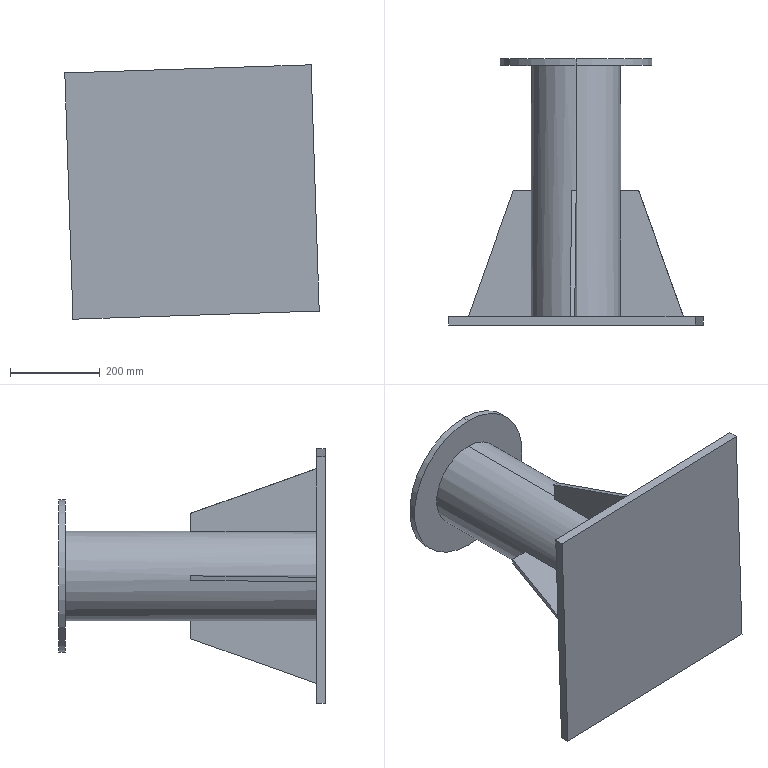Part | SolidWorks | features BaseBody 1 | 1 solid | 28 faces | box 567.987 x 595 x 567.987 mm | volume 26013266 mm3 | plane 24 | cylinder 4 | commonest cylinder face diameters 200 x2 340 x2
STEP:
#1=CARTESIAN_POINT('',(-1049.138,-596.769,-2188.931));
#2=VERTEX_POINT('',#1);
#3=CARTESIAN_POINT('',(-1049.138,-596.769,-1988.931));
#4=VERTEX_POINT('',#3);
#5=CARTESIAN_POINT('',(-1049.138,-596.769,-2088.931));
#6=DIRECTION('',(0.,-1.,0.));
#7=DIRECTION('',(0.,0.,-1.));
#8=AXIS2_PLACEMENT_3D('',#5,#6,#7);
#9=CIRCLE('',#8,100.);
#10=EDGE_CURVE('',#2,#4,#9,.T.);
#11=ORIENTED_EDGE('',*,*,#10,.T.);
#12=CARTESIAN_POINT('',(-1049.138,-876.769,-1988.931));
#13=VERTEX_POINT('',#12);
#14=CARTESIAN_POINT('',(-1049.138,-596.769,-1988.931));
#15=DIRECTION('',(0.,-1.,0.));
#16=VECTOR('',#15,1000.);
#17=LINE('',#14,#16);
#18=EDGE_CURVE('',#4,#13,#17,.T.);
#19=ORIENTED_EDGE('',*,*,#18,.T.);
#20=CARTESIAN_POINT('',(-1047.462,-876.769,-1988.945));
#21=VERTEX_POINT('',#20);
#22=CARTESIAN_POINT('',(-1049.138,-876.769,-2088.931));
#23=DIRECTION('',(0.,1.,0.));
#24=DIRECTION('',(0.,0.,-1.));
#25=AXIS2_PLACEMENT_3D('',#22,#23,#24);
#26=CIRCLE('',#25,100.);
#27=EDGE_CURVE('',#13,#21,#26,.T.);
#28=ORIENTED_EDGE('',*,*,#27,.T.);
#29=CARTESIAN_POINT('',(-1047.462,-1156.769,-1988.945));
#30=VERTEX_POINT('',#29);
#31=CARTESIAN_POINT('',(-1047.462,-596.769,-1988.945));
#32=DIRECTION('',(0.,-1.,0.));
#33=VECTOR('',#32,1000.);
#34=LINE('',#31,#33);
#35=EDGE_CURVE('',#21,#30,#34,.T.);
#36=ORIENTED_EDGE('',*,*,#35,.T.);
#37=CARTESIAN_POINT('',(-949.485,-1156.769,-2080.612));
#38=VERTEX_POINT('',#37);
#39=CARTESIAN_POINT('',(-1049.138,-1156.769,-2088.931));
#40=DIRECTION('',(0.,-1.,0.));
#41=DIRECTION('',(0.,0.,-1.));
#42=AXIS2_PLACEMENT_3D('',#39,#40,#41);
#43=CIRCLE('',#42,100.);
#44=EDGE_CURVE('',#38,#30,#43,.T.);
#45=ORIENTED_EDGE('',*,*,#44,.F.);
#46=CARTESIAN_POINT('',(-949.485,-876.769,-2080.612));
#47=VERTEX_POINT('',#46);
#48=CARTESIAN_POINT('',(-949.485,-596.769,-2080.612));
#49=DIRECTION('',(0.,1.,0.));
#50=VECTOR('',#49,1000.);
#51=LINE('',#48,#50);
#52=EDGE_CURVE('',#38,#47,#51,.T.);
#53=ORIENTED_EDGE('',*,*,#52,.T.);
#54=CARTESIAN_POINT('',(-949.152,-876.769,-2090.607));
#55=VERTEX_POINT('',#54);
#56=CARTESIAN_POINT('',(-1049.138,-876.769,-2088.931));
#57=DIRECTION('',(0.,1.,0.));
#58=DIRECTION('',(0.,0.,-1.));
#59=AXIS2_PLACEMENT_3D('',#56,#57,#58);
#60=CIRCLE('',#59,100.);
#61=EDGE_CURVE('',#47,#55,#60,.T.);
#62=ORIENTED_EDGE('',*,*,#61,.T.);
#63=CARTESIAN_POINT('',(-949.152,-1156.769,-2090.607));
#64=VERTEX_POINT('',#63);
#65=CARTESIAN_POINT('',(-949.152,-596.769,-2090.607));
#66=DIRECTION('',(0.,-1.,0.));
#67=VECTOR('',#66,1000.);
#68=LINE('',#65,#67);
#69=EDGE_CURVE('',#55,#64,#68,.T.);
#70=ORIENTED_EDGE('',*,*,#69,.T.);
#71=CARTESIAN_POINT('',(-1040.819,-1156.769,-2188.585));
#72=VERTEX_POINT('',#71);
#73=CARTESIAN_POINT('',(-1049.138,-1156.769,-2088.931));
#74=DIRECTION('',(0.,-1.,0.));
#75=DIRECTION('',(0.,0.,-1.));
#76=AXIS2_PLACEMENT_3D('',#73,#74,#75);
#77=CIRCLE('',#76,100.);
#78=EDGE_CURVE('',#72,#64,#77,.T.);
#79=ORIENTED_EDGE('',*,*,#78,.F.);
#80=CARTESIAN_POINT('',(-1040.819,-876.769,-2188.585));
#81=VERTEX_POINT('',#80);
#82=CARTESIAN_POINT('',(-1040.819,-596.769,-2188.585));
#83=DIRECTION('',(0.,1.,0.));
#84=VECTOR('',#83,1000.);
#85=LINE('',#82,#84);
#86=EDGE_CURVE('',#72,#81,#85,.T.);
#87=ORIENTED_EDGE('',*,*,#86,.T.);
#88=CARTESIAN_POINT('',(-1049.138,-876.769,-2188.931));
#89=VERTEX_POINT('',#88);
#90=CARTESIAN_POINT('',(-1049.138,-876.769,-2088.931));
#91=DIRECTION('',(0.,1.,0.));
#92=DIRECTION('',(0.,0.,-1.));
#93=AXIS2_PLACEMENT_3D('',#90,#91,#92);
#94=CIRCLE('',#93,100.);
#95=EDGE_CURVE('',#81,#89,#94,.T.);
#96=ORIENTED_EDGE('',*,*,#95,.T.);
#97=CARTESIAN_POINT('',(-1049.138,-596.769,-2188.931));
#98=DIRECTION('',(0.,-1.,0.));
#99=VECTOR('',#98,1000.);
#100=LINE('',#97,#99);
#101=EDGE_CURVE('',#2,#89,#100,.T.);
#102=ORIENTED_EDGE('',*,*,#101,.F.);
#103=EDGE_LOOP('',(#11,#19,#28,#36,#45,#53,#62,#70,#79,#87,#96,#102));
#104=FACE_OUTER_BOUND('',#103,.T.);
#105=CARTESIAN_POINT('',(-1049.138,-596.769,-2088.931));
#106=DIRECTION('',(0.,-1.,0.));
#107=DIRECTION('',(0.,0.,-1.));
#108=AXIS2_PLACEMENT_3D('',#105,#106,#107);
#109=CYLINDRICAL_SURFACE('',#108,100.);
#110=ADVANCED_FACE('',(#104),#109,.T.);
#111=CARTESIAN_POINT('',(-1049.138,-581.769,-2258.931));
#112=VERTEX_POINT('',#111);
#113=CARTESIAN_POINT('',(-1049.138,-581.769,-1918.931));
#114=VERTEX_POINT('',#113);
#115=CARTESIAN_POINT('',(-1049.138,-581.769,-2088.931));
#116=DIRECTION('',(0.,-1.,0.));
#117=DIRECTION('',(0.,0.,-1.));
#118=AXIS2_PLACEMENT_3D('',#115,#116,#117);
#119=CIRCLE('',#118,170.);
#120=EDGE_CURVE('',#112,#114,#119,.T.);
#121=ORIENTED_EDGE('',*,*,#120,.T.);
#122=CARTESIAN_POINT('',(-1049.138,-596.769,-1918.931));
#123=VERTEX_POINT('',#122);
#124=CARTESIAN_POINT('',(-1049.138,-581.769,-1918.931));
#125=DIRECTION('',(0.,-1.,0.));
#126=VECTOR('',#125,1000.);
#127=LINE('',#124,#126);
#128=EDGE_CURVE('',#114,#123,#127,.T.);
#129=ORIENTED_EDGE('',*,*,#128,.T.);
#130=CARTESIAN_POINT('',(-1049.138,-596.769,-2258.931));
#131=VERTEX_POINT('',#130);
#132=CARTESIAN_POINT('',(-1049.138,-596.769,-2088.931));
#133=DIRECTION('',(0.,1.,0.));
#134=DIRECTION('',(0.,0.,-1.));
#135=AXIS2_PLACEMENT_3D('',#132,#133,#134);
#136=CIRCLE('',#135,170.);
#137=EDGE_CURVE('',#123,#131,#136,.T.);
#138=ORIENTED_EDGE('',*,*,#137,.T.);
#139=CARTESIAN_POINT('',(-1049.138,-581.769,-2258.931));
#140=DIRECTION('',(0.,-1.,0.));
#141=VECTOR('',#140,1000.);
#142=LINE('',#139,#141);
#143=EDGE_CURVE('',#112,#131,#142,.T.);
#144=ORIENTED_EDGE('',*,*,#143,.F.);
#145=EDGE_LOOP('',(#121,#129,#138,#144));
#146=FACE_OUTER_BOUND('',#145,.T.);
#147=CARTESIAN_POINT('',(-1049.138,-581.769,-2088.931));
#148=DIRECTION('',(0.,-1.,0.));
#149=DIRECTION('',(0.,0.,-1.));
#150=AXIS2_PLACEMENT_3D('',#147,#148,#149);
#151=CYLINDRICAL_SURFACE('',#150,170.);
#152=ADVANCED_FACE('',(#146),#151,.T.);
#153=CARTESIAN_POINT('',(-765.144,-1176.769,-2354.633));
#154=VERTEX_POINT('',#153);
#155=CARTESIAN_POINT('',(-1314.84,-1176.769,-2372.925));
#156=VERTEX_POINT('',#155);
#157=CARTESIAN_POINT('',(-765.144,-1176.769,-2354.633));
#158=DIRECTION('',(-0.9994,0.,-0.03326));
#159=VECTOR('',#158,1000.);
#160=LINE('',#157,#159);
#161=EDGE_CURVE('',#154,#156,#160,.T.);
#162=ORIENTED_EDGE('',*,*,#161,.F.);
#163=CARTESIAN_POINT('',(-783.436,-1176.769,-1804.938));
#164=VERTEX_POINT('',#163);
#165=CARTESIAN_POINT('',(-783.436,-1176.769,-1804.938));
#166=DIRECTION('',(0.03326,0.,-0.9994));
#167=VECTOR('',#166,1000.);
#168=LINE('',#165,#167);
#169=EDGE_CURVE('',#164,#154,#168,.T.);
#170=ORIENTED_EDGE('',*,*,#169,.F.);
#171=CARTESIAN_POINT('',(-1333.132,-1176.769,-1823.229));
#172=VERTEX_POINT('',#171);
#173=CARTESIAN_POINT('',(-1333.132,-1176.769,-1823.229));
#174=DIRECTION('',(0.9994,0.,0.03326));
#175=VECTOR('',#174,1000.);
#176=LINE('',#173,#175);
#177=EDGE_CURVE('',#172,#164,#176,.T.);
#178=ORIENTED_EDGE('',*,*,#177,.F.);
#179=CARTESIAN_POINT('',(-1314.84,-1176.769,-2372.925));
#180=DIRECTION('',(-0.03326,0.,0.9994));
#181=VECTOR('',#180,1000.);
#182=LINE('',#179,#181);
#183=EDGE_CURVE('',#156,#172,#182,.T.);
#184=ORIENTED_EDGE('',*,*,#183,.F.);
#185=EDGE_LOOP('',(#162,#170,#178,#184));
#186=FACE_OUTER_BOUND('',#185,.T.);
#187=CARTESIAN_POINT('',(-1049.138,-1176.769,-2088.931));
#188=DIRECTION('',(0.,1.,0.));
#189=DIRECTION('',(0.,0.,1.));
#190=AXIS2_PLACEMENT_3D('',#187,#188,#189);
#191=PLANE('',#190);
#192=ADVANCED_FACE('',(#186),#191,.F.);
#193=CARTESIAN_POINT('',(-1333.132,-1156.769,-1823.229));
#194=VERTEX_POINT('',#193);
#195=CARTESIAN_POINT('',(-1333.132,-1156.769,-1823.229));
#196=DIRECTION('',(0.,-1.,0.));
#197=VECTOR('',#196,1000.);
#198=LINE('',#195,#197);
#199=EDGE_CURVE('',#194,#172,#198,.T.);
#200=ORIENTED_EDGE('',*,*,#199,.F.);
#201=CARTESIAN_POINT('',(-1314.84,-1156.769,-2372.925));
#202=VERTEX_POINT('',#201);
#203=CARTESIAN_POINT('',(-1314.84,-1156.769,-2372.925));
#204=DIRECTION('',(-0.03326,0.,0.9994));
#205=VECTOR('',#204,1000.);
#206=LINE('',#203,#205);
#207=EDGE_CURVE('',#202,#194,#206,.T.);
#208=ORIENTED_EDGE('',*,*,#207,.F.);
#209=CARTESIAN_POINT('',(-1314.84,-1156.769,-2372.925));
#210=DIRECTION('',(0.,1.,0.));
#211=VECTOR('',#210,1000.);
#212=LINE('',#209,#211);
#213=EDGE_CURVE('',#156,#202,#212,.T.);
#214=ORIENTED_EDGE('',*,*,#213,.F.);
#215=ORIENTED_EDGE('',*,*,#183,.T.);
#216=EDGE_LOOP('',(#200,#208,#214,#215));
#217=FACE_OUTER_BOUND('',#216,.T.);
#218=CARTESIAN_POINT('',(-1314.84,-1156.769,-2372.925));
#219=DIRECTION('',(0.9994,0.,0.03326));
#220=DIRECTION('',(0.03326,0.,-0.9994));
#221=AXIS2_PLACEMENT_3D('',#218,#219,#220);
#222=PLANE('',#221);
#223=ADVANCED_FACE('',(#217),#222,.F.);
#224=ORIENTED_EDGE('',*,*,#213,.T.);
#225=CARTESIAN_POINT('',(-765.144,-1156.769,-2354.633));
#226=VERTEX_POINT('',#225);
#227=CARTESIAN_POINT('',(-1314.84,-1156.769,-2372.925));
#228=DIRECTION('',(-0.9994,0.,-0.03326));
#229=VECTOR('',#228,1000.);
#230=LINE('',#227,#229);
#231=EDGE_CURVE('',#226,#202,#230,.T.);
#232=ORIENTED_EDGE('',*,*,#231,.F.);
#233=CARTESIAN_POINT('',(-765.144,-1156.769,-2354.633));
#234=DIRECTION('',(0.,1.,0.));
#235=VECTOR('',#234,1000.);
#236=LINE('',#233,#235);
#237=EDGE_CURVE('',#154,#226,#236,.T.);
#238=ORIENTED_EDGE('',*,*,#237,.F.);
#239=ORIENTED_EDGE('',*,*,#161,.T.);
#240=EDGE_LOOP('',(#224,#232,#238,#239));
#241=FACE_OUTER_BOUND('',#240,.T.);
#242=CARTESIAN_POINT('',(-1314.84,-1156.769,-2372.925));
#243=DIRECTION('',(-0.03326,0.,0.9994));
#244=DIRECTION('',(0.9994,0.,0.03326));
#245=AXIS2_PLACEMENT_3D('',#242,#243,#244);
#246=PLANE('',#245);
#247=ADVANCED_FACE('',(#241),#246,.F.);
#248=ORIENTED_EDGE('',*,*,#237,.T.);
#249=CARTESIAN_POINT('',(-783.436,-1156.769,-1804.938));
#250=VERTEX_POINT('',#249);
#251=CARTESIAN_POINT('',(-765.144,-1156.769,-2354.633));
#252=DIRECTION('',(0.03326,0.,-0.9994));
#253=VECTOR('',#252,1000.);
#254=LINE('',#251,#253);
#255=EDGE_CURVE('',#250,#226,#254,.T.);
#256=ORIENTED_EDGE('',*,*,#255,.F.);
#257=CARTESIAN_POINT('',(-783.436,-1156.769,-1804.938));
#258=DIRECTION('',(0.,1.,0.));
#259=VECTOR('',#258,1000.);
#260=LINE('',#257,#259);
#261=EDGE_CURVE('',#164,#250,#260,.T.);
#262=ORIENTED_EDGE('',*,*,#261,.F.);
#263=ORIENTED_EDGE('',*,*,#169,.T.);
#264=EDGE_LOOP('',(#248,#256,#262,#263));
#265=FACE_OUTER_BOUND('',#264,.T.);
#266=CARTESIAN_POINT('',(-765.144,-1156.769,-2354.633));
#267=DIRECTION('',(-0.9994,0.,-0.03326));
#268=DIRECTION('',(-0.03326,0.,0.9994));
#269=AXIS2_PLACEMENT_3D('',#266,#267,#268);
#270=PLANE('',#269);
#271=ADVANCED_FACE('',(#265),#270,.F.);
#272=ORIENTED_EDGE('',*,*,#261,.T.);
#273=CARTESIAN_POINT('',(-1333.132,-1156.769,-1823.229));
#274=DIRECTION('',(0.9994,0.,0.03326));
#275=VECTOR('',#274,1000.);
#276=LINE('',#273,#275);
#277=EDGE_CURVE('',#194,#250,#276,.T.);
#278=ORIENTED_EDGE('',*,*,#277,.F.);
#279=ORIENTED_EDGE('',*,*,#199,.T.);
#280=ORIENTED_EDGE('',*,*,#177,.T.);
#281=EDGE_LOOP('',(#272,#278,#279,#280));
#282=FACE_OUTER_BOUND('',#281,.T.);
#283=CARTESIAN_POINT('',(-1333.132,-1156.769,-1823.229));
#284=DIRECTION('',(0.03326,0.,-0.9994));
#285=DIRECTION('',(-0.9994,0.,-0.03326));
#286=AXIS2_PLACEMENT_3D('',#283,#284,#285);
#287=PLANE('',#286);
#288=ADVANCED_FACE('',(#282),#287,.F.);
#289=CARTESIAN_POINT('',(-1148.791,-1156.769,-2097.25));
#290=VERTEX_POINT('',#289);
#291=CARTESIAN_POINT('',(-1050.814,-1156.769,-2188.917));
#292=VERTEX_POINT('',#291);
#293=CARTESIAN_POINT('',(-1049.138,-1156.769,-2088.931));
#294=DIRECTION('',(0.,-1.,0.));
#295=DIRECTION('',(0.,0.,-1.));
#296=AXIS2_PLACEMENT_3D('',#293,#294,#295);
#297=CIRCLE('',#296,100.);
#298=EDGE_CURVE('',#290,#292,#297,.T.);
#299=ORIENTED_EDGE('',*,*,#298,.T.);
#300=CARTESIAN_POINT('',(-1046.153,-1156.769,-2328.965));
#301=VERTEX_POINT('',#300);
#302=CARTESIAN_POINT('',(-1050.814,-1156.769,-2188.917));
#303=DIRECTION('',(0.03326,0.,-0.9994));
#304=VECTOR('',#303,1000.);
#305=LINE('',#302,#304);
#306=EDGE_CURVE('',#292,#301,#305,.T.);
#307=ORIENTED_EDGE('',*,*,#306,.T.);
#308=CARTESIAN_POINT('',(-1036.159,-1156.769,-2328.632));
#309=VERTEX_POINT('',#308);
#310=CARTESIAN_POINT('',(-1046.153,-1156.769,-2328.965));
#311=DIRECTION('',(0.9994,0.,0.03326));
#312=VECTOR('',#311,1000.);
#313=LINE('',#310,#312);
#314=EDGE_CURVE('',#301,#309,#313,.T.);
#315=ORIENTED_EDGE('',*,*,#314,.T.);
#316=CARTESIAN_POINT('',(-1036.159,-1156.769,-2328.632));
#317=DIRECTION('',(-0.03326,0.,0.9994));
#318=VECTOR('',#317,1000.);
#319=LINE('',#316,#318);
#320=EDGE_CURVE('',#309,#72,#319,.T.);
#321=ORIENTED_EDGE('',*,*,#320,.T.);
#322=ORIENTED_EDGE('',*,*,#78,.T.);
#323=CARTESIAN_POINT('',(-809.104,-1156.769,-2085.947));
#324=VERTEX_POINT('',#323);
#325=CARTESIAN_POINT('',(-949.152,-1156.769,-2090.607));
#326=DIRECTION('',(0.9994,0.,0.03326));
#327=VECTOR('',#326,1000.);
#328=LINE('',#325,#327);
#329=EDGE_CURVE('',#64,#324,#328,.T.);
#330=ORIENTED_EDGE('',*,*,#329,.T.);
#331=CARTESIAN_POINT('',(-809.437,-1156.769,-2075.952));
#332=VERTEX_POINT('',#331);
#333=CARTESIAN_POINT('',(-809.104,-1156.769,-2085.947));
#334=DIRECTION('',(-0.03326,0.,0.9994));
#335=VECTOR('',#334,1000.);
#336=LINE('',#333,#335);
#337=EDGE_CURVE('',#324,#332,#336,.T.);
#338=ORIENTED_EDGE('',*,*,#337,.T.);
#339=CARTESIAN_POINT('',(-809.437,-1156.769,-2075.952));
#340=DIRECTION('',(-0.9994,0.,-0.03326));
#341=VECTOR('',#340,1000.);
#342=LINE('',#339,#341);
#343=EDGE_CURVE('',#332,#38,#342,.T.);
#344=ORIENTED_EDGE('',*,*,#343,.T.);
#345=ORIENTED_EDGE('',*,*,#44,.T.);
#346=CARTESIAN_POINT('',(-1052.123,-1156.769,-1848.898));
#347=VERTEX_POINT('',#346);
#348=CARTESIAN_POINT('',(-1047.462,-1156.769,-1988.945));
#349=DIRECTION('',(-0.03326,0.,0.9994));
#350=VECTOR('',#349,1000.);
#351=LINE('',#348,#350);
#352=EDGE_CURVE('',#30,#347,#351,.T.);
#353=ORIENTED_EDGE('',*,*,#352,.T.);
#354=CARTESIAN_POINT('',(-1062.117,-1156.769,-1849.23));
#355=VERTEX_POINT('',#354);
#356=CARTESIAN_POINT('',(-1052.123,-1156.769,-1848.898));
#357=DIRECTION('',(-0.9994,0.,-0.03326));
#358=VECTOR('',#357,1000.);
#359=LINE('',#356,#358);
#360=EDGE_CURVE('',#347,#355,#359,.T.);
#361=ORIENTED_EDGE('',*,*,#360,.T.);
#362=CARTESIAN_POINT('',(-1057.457,-1156.769,-1989.278));
#363=VERTEX_POINT('',#362);
#364=CARTESIAN_POINT('',(-1062.117,-1156.769,-1849.23));
#365=DIRECTION('',(0.03326,0.,-0.9994));
#366=VECTOR('',#365,1000.);
#367=LINE('',#364,#366);
#368=EDGE_CURVE('',#355,#363,#367,.T.);
#369=ORIENTED_EDGE('',*,*,#368,.T.);
#370=CARTESIAN_POINT('',(-1149.124,-1156.769,-2087.256));
#371=VERTEX_POINT('',#370);
#372=CARTESIAN_POINT('',(-1049.138,-1156.769,-2088.931));
#373=DIRECTION('',(0.,-1.,0.));
#374=DIRECTION('',(0.,0.,-1.));
#375=AXIS2_PLACEMENT_3D('',#372,#373,#374);
#376=CIRCLE('',#375,100.);
#377=EDGE_CURVE('',#363,#371,#376,.T.);
#378=ORIENTED_EDGE('',*,*,#377,.T.);
#379=CARTESIAN_POINT('',(-1289.171,-1156.769,-2091.916));
#380=VERTEX_POINT('',#379);
#381=CARTESIAN_POINT('',(-1149.124,-1156.769,-2087.256));
#382=DIRECTION('',(-0.9994,0.,-0.03326));
#383=VECTOR('',#382,1000.);
#384=LINE('',#381,#383);
#385=EDGE_CURVE('',#371,#380,#384,.T.);
#386=ORIENTED_EDGE('',*,*,#385,.T.);
#387=CARTESIAN_POINT('',(-1288.839,-1156.769,-2101.91));
#388=VERTEX_POINT('',#387);
#389=CARTESIAN_POINT('',(-1289.171,-1156.769,-2091.916));
#390=DIRECTION('',(0.03326,0.,-0.9994));
#391=VECTOR('',#390,1000.);
#392=LINE('',#389,#391);
#393=EDGE_CURVE('',#380,#388,#392,.T.);
#394=ORIENTED_EDGE('',*,*,#393,.T.);
#395=CARTESIAN_POINT('',(-1288.839,-1156.769,-2101.91));
#396=DIRECTION('',(0.9994,0.,0.03326));
#397=VECTOR('',#396,1000.);
#398=LINE('',#395,#397);
#399=EDGE_CURVE('',#388,#290,#398,.T.);
#400=ORIENTED_EDGE('',*,*,#399,.T.);
#401=EDGE_LOOP('',(#299,#307,#315,#321,#322,#330,#338,#344,#345,#353,#361,#369,#378,#386,#394,#400));
#402=FACE_BOUND('',#401,.T.);
#403=ORIENTED_EDGE('',*,*,#277,.T.);
#404=ORIENTED_EDGE('',*,*,#255,.T.);
#405=ORIENTED_EDGE('',*,*,#231,.T.);
#406=ORIENTED_EDGE('',*,*,#207,.T.);
#407=EDGE_LOOP('',(#403,#404,#405,#406));
#408=FACE_OUTER_BOUND('',#407,.T.);
#409=CARTESIAN_POINT('',(-1049.138,-1156.769,-2088.931));
#410=DIRECTION('',(0.,1.,0.));
#411=DIRECTION('',(0.,0.,1.));
#412=AXIS2_PLACEMENT_3D('',#409,#410,#411);
#413=PLANE('',#412);
#414=ADVANCED_FACE('',(#402,#408),#413,.T.);
#415=CARTESIAN_POINT('',(-1050.814,-876.769,-2188.917));
#416=VERTEX_POINT('',#415);
#417=CARTESIAN_POINT('',(-1050.814,-879.269,-2188.917));
#418=DIRECTION('',(0.,1.,0.));
#419=VECTOR('',#418,1000.);
#420=LINE('',#417,#419);
#421=EDGE_CURVE('',#292,#416,#420,.T.);
#422=ORIENTED_EDGE('',*,*,#421,.T.);
#423=CARTESIAN_POINT('',(-1049.479,-876.769,-2229.02));
#424=VERTEX_POINT('',#423);
#425=CARTESIAN_POINT('',(-1054.135,-876.769,-2089.098));
#426=DIRECTION('',(0.03326,0.,-0.9994));
#427=VECTOR('',#426,1000.);
#428=LINE('',#425,#427);
#429=EDGE_CURVE('',#416,#424,#428,.T.);
#430=ORIENTED_EDGE('',*,*,#429,.T.);
#431=CARTESIAN_POINT('',(-1049.479,-876.769,-2229.02));
#432=DIRECTION('',(0.01119,-0.9417,-0.3362));
#433=VECTOR('',#432,1000.);
#434=LINE('',#431,#433);
#435=EDGE_CURVE('',#424,#301,#434,.T.);
#436=ORIENTED_EDGE('',*,*,#435,.T.);
#437=ORIENTED_EDGE('',*,*,#306,.F.);
#438=EDGE_LOOP('',(#422,#430,#436,#437));
#439=FACE_OUTER_BOUND('',#438,.T.);
#440=CARTESIAN_POINT('',(-1054.135,-879.269,-2089.098));
#441=DIRECTION('',(-0.9994,0.,-0.03326));
#442=DIRECTION('',(-0.03326,0.,0.9994));
#443=AXIS2_PLACEMENT_3D('',#440,#441,#442);
#444=PLANE('',#443);
#445=ADVANCED_FACE('',(#439),#444,.T.);
#446=ORIENTED_EDGE('',*,*,#18,.F.);
#447=CARTESIAN_POINT('',(-1049.138,-596.769,-2088.931));
#448=DIRECTION('',(0.,-1.,0.));
#449=DIRECTION('',(0.,0.,-1.));
#450=AXIS2_PLACEMENT_3D('',#447,#448,#449);
#451=CIRCLE('',#450,100.);
#452=EDGE_CURVE('',#4,#2,#451,.T.);
#453=ORIENTED_EDGE('',*,*,#452,.T.);
#454=ORIENTED_EDGE('',*,*,#101,.T.);
#455=CARTESIAN_POINT('',(-1049.138,-876.769,-2088.931));
#456=DIRECTION('',(0.,1.,0.));
#457=DIRECTION('',(0.,0.,-1.));
#458=AXIS2_PLACEMENT_3D('',#455,#456,#457);
#459=CIRCLE('',#458,100.);
#460=EDGE_CURVE('',#89,#416,#459,.T.);
#461=ORIENTED_EDGE('',*,*,#460,.T.);
#462=ORIENTED_EDGE('',*,*,#421,.F.);
#463=ORIENTED_EDGE('',*,*,#298,.F.);
#464=CARTESIAN_POINT('',(-1148.791,-876.769,-2097.25));
#465=VERTEX_POINT('',#464);
#466=CARTESIAN_POINT('',(-1148.791,-596.769,-2097.25));
#467=DIRECTION('',(0.,1.,0.));
#468=VECTOR('',#467,1000.);
#469=LINE('',#466,#468);
#470=EDGE_CURVE('',#290,#465,#469,.T.);
#471=ORIENTED_EDGE('',*,*,#470,.T.);
#472=CARTESIAN_POINT('',(-1149.124,-876.769,-2087.256));
#473=VERTEX_POINT('',#472);
#474=CARTESIAN_POINT('',(-1049.138,-876.769,-2088.931));
#475=DIRECTION('',(0.,1.,0.));
#476=DIRECTION('',(0.,0.,-1.));
#477=AXIS2_PLACEMENT_3D('',#474,#475,#476);
#478=CIRCLE('',#477,100.);
#479=EDGE_CURVE('',#465,#473,#478,.T.);
#480=ORIENTED_EDGE('',*,*,#479,.T.);
#481=CARTESIAN_POINT('',(-1149.124,-596.769,-2087.256));
#482=DIRECTION('',(0.,-1.,0.));
#483=VECTOR('',#482,1000.);
#484=LINE('',#481,#483);
#485=EDGE_CURVE('',#473,#371,#484,.T.);
#486=ORIENTED_EDGE('',*,*,#485,.T.);
#487=ORIENTED_EDGE('',*,*,#377,.F.);
#488=CARTESIAN_POINT('',(-1057.457,-876.769,-1989.278));
#489=VERTEX_POINT('',#488);
#490=CARTESIAN_POINT('',(-1057.457,-596.769,-1989.278));
#491=DIRECTION('',(0.,1.,0.));
#492=VECTOR('',#491,1000.);
#493=LINE('',#490,#492);
#494=EDGE_CURVE('',#363,#489,#493,.T.);
#495=ORIENTED_EDGE('',*,*,#494,.T.);
#496=CARTESIAN_POINT('',(-1049.138,-876.769,-2088.931));
#497=DIRECTION('',(0.,1.,0.));
#498=DIRECTION('',(0.,0.,-1.));
#499=AXIS2_PLACEMENT_3D('',#496,#497,#498);
#500=CIRCLE('',#499,100.);
#501=EDGE_CURVE('',#489,#13,#500,.T.);
#502=ORIENTED_EDGE('',*,*,#501,.T.);
#503=EDGE_LOOP('',(#446,#453,#454,#461,#462,#463,#471,#480,#486,#487,#495,#502));
#504=FACE_OUTER_BOUND('',#503,.T.);
#505=CARTESIAN_POINT('',(-1049.138,-596.769,-2088.931));
#506=DIRECTION('',(0.,-1.,0.));
#507=DIRECTION('',(0.,0.,-1.));
#508=AXIS2_PLACEMENT_3D('',#505,#506,#507);
#509=CYLINDRICAL_SURFACE('',#508,100.);
#510=ADVANCED_FACE('',(#504),#509,.T.);
#511=CARTESIAN_POINT('',(-1188.894,-876.769,-2098.585));
#512=VERTEX_POINT('',#511);
#513=CARTESIAN_POINT('',(-1188.894,-876.769,-2098.585));
#514=DIRECTION('',(-0.3362,-0.9417,-0.01119));
#515=VECTOR('',#514,1000.);
#516=LINE('',#513,#515);
#517=EDGE_CURVE('',#512,#388,#516,.T.);
#518=ORIENTED_EDGE('',*,*,#517,.F.);
#519=CARTESIAN_POINT('',(-1048.972,-876.769,-2093.928));
#520=DIRECTION('',(-0.9994,0.,-0.03326));
#521=VECTOR('',#520,1000.);
#522=LINE('',#519,#521);
#523=EDGE_CURVE('',#465,#512,#522,.T.);
#524=ORIENTED_EDGE('',*,*,#523,.F.);
#525=ORIENTED_EDGE('',*,*,#470,.F.);
#526=ORIENTED_EDGE('',*,*,#399,.F.);
#527=EDGE_LOOP('',(#518,#524,#525,#526));
#528=FACE_OUTER_BOUND('',#527,.T.);
#529=CARTESIAN_POINT('',(-1048.972,-879.269,-2093.928));
#530=DIRECTION('',(-0.03326,0.,0.9994));
#531=DIRECTION('',(0.9994,0.,0.03326));
#532=AXIS2_PLACEMENT_3D('',#529,#530,#531);
#533=PLANE('',#532);
#534=ADVANCED_FACE('',(#528),#533,.F.);
#535=CARTESIAN_POINT('',(-1189.227,-876.769,-2088.59));
#536=VERTEX_POINT('',#535);
#537=CARTESIAN_POINT('',(-1289.171,-1156.769,-2091.916));
#538=DIRECTION('',(0.3362,0.9417,0.01119));
#539=VECTOR('',#538,1000.);
#540=LINE('',#537,#539);
#541=EDGE_CURVE('',#380,#536,#540,.T.);
#542=ORIENTED_EDGE('',*,*,#541,.T.);
#543=CARTESIAN_POINT('',(-1189.227,-876.769,-2088.59));
#544=DIRECTION('',(0.03326,0.,-0.9994));
#545=VECTOR('',#544,1000.);
#546=LINE('',#543,#545);
#547=EDGE_CURVE('',#536,#512,#546,.T.);
#548=ORIENTED_EDGE('',*,*,#547,.T.);
#549=ORIENTED_EDGE('',*,*,#517,.T.);
#550=ORIENTED_EDGE('',*,*,#393,.F.);
#551=EDGE_LOOP('',(#542,#548,#549,#550));
#552=FACE_OUTER_BOUND('',#551,.T.);
#553=CARTESIAN_POINT('',(-1189.06,-876.769,-2093.587));
#554=DIRECTION('',(-0.9412,0.3363,-0.03132));
#555=DIRECTION('',(-0.3365,-0.9417,0.));
#556=AXIS2_PLACEMENT_3D('',#553,#554,#555);
#557=PLANE('',#556);
#558=ADVANCED_FACE('',(#552),#557,.T.);
#559=ORIENTED_EDGE('',*,*,#485,.F.);
#560=CARTESIAN_POINT('',(-1049.304,-876.769,-2083.934));
#561=DIRECTION('',(-0.9994,0.,-0.03326));
#562=VECTOR('',#561,1000.);
#563=LINE('',#560,#562);
#564=EDGE_CURVE('',#473,#536,#563,.T.);
#565=ORIENTED_EDGE('',*,*,#564,.T.);
#566=ORIENTED_EDGE('',*,*,#541,.F.);
#567=ORIENTED_EDGE('',*,*,#385,.F.);
#568=EDGE_LOOP('',(#559,#565,#566,#567));
#569=FACE_OUTER_BOUND('',#568,.T.);
#570=CARTESIAN_POINT('',(-1049.304,-879.269,-2083.934));
#571=DIRECTION('',(-0.03326,0.,0.9994));
#572=DIRECTION('',(0.9994,0.,0.03326));
#573=AXIS2_PLACEMENT_3D('',#570,#571,#572);
#574=PLANE('',#573);
#575=ADVANCED_FACE('',(#569),#574,.T.);
#576=CARTESIAN_POINT('',(-1058.791,-876.769,-1949.175));
#577=VERTEX_POINT('',#576);
#578=CARTESIAN_POINT('',(-1058.791,-876.769,-1949.175));
#579=DIRECTION('',(-0.01119,-0.9417,0.3362));
#580=VECTOR('',#579,1000.);
#581=LINE('',#578,#580);
#582=EDGE_CURVE('',#577,#355,#581,.T.);
#583=ORIENTED_EDGE('',*,*,#582,.F.);
#584=CARTESIAN_POINT('',(-1054.135,-876.769,-2089.098));
#585=DIRECTION('',(-0.03326,0.,0.9994));
#586=VECTOR('',#585,1000.);
#587=LINE('',#584,#586);
#588=EDGE_CURVE('',#489,#577,#587,.T.);
#589=ORIENTED_EDGE('',*,*,#588,.F.);
#590=ORIENTED_EDGE('',*,*,#494,.F.);
#591=ORIENTED_EDGE('',*,*,#368,.F.);
#592=EDGE_LOOP('',(#583,#589,#590,#591));
#593=FACE_OUTER_BOUND('',#592,.T.);
#594=CARTESIAN_POINT('',(-1054.135,-879.269,-2089.098));
#595=DIRECTION('',(0.9994,0.,0.03326));
#596=DIRECTION('',(0.03326,0.,-0.9994));
#597=AXIS2_PLACEMENT_3D('',#594,#595,#596);
#598=PLANE('',#597);
#599=ADVANCED_FACE('',(#593),#598,.F.);
#600=CARTESIAN_POINT('',(-1048.797,-876.769,-1948.842));
#601=VERTEX_POINT('',#600);
#602=CARTESIAN_POINT('',(-1052.123,-1156.769,-1848.898));
#603=DIRECTION('',(0.01119,0.9417,-0.3362));
#604=VECTOR('',#603,1000.);
#605=LINE('',#602,#604);
#606=EDGE_CURVE('',#347,#601,#605,.T.);
#607=ORIENTED_EDGE('',*,*,#606,.T.);
#608=CARTESIAN_POINT('',(-1048.797,-876.769,-1948.842));
#609=DIRECTION('',(-0.9994,0.,-0.03326));
#610=VECTOR('',#609,1000.);
#611=LINE('',#608,#610);
#612=EDGE_CURVE('',#601,#577,#611,.T.);
#613=ORIENTED_EDGE('',*,*,#612,.T.);
#614=ORIENTED_EDGE('',*,*,#582,.T.);
#615=ORIENTED_EDGE('',*,*,#360,.F.);
#616=EDGE_LOOP('',(#607,#613,#614,#615));
#617=FACE_OUTER_BOUND('',#616,.T.);
#618=CARTESIAN_POINT('',(-1053.794,-876.769,-1949.009));
#619=DIRECTION('',(-0.03132,0.3363,0.9412));
#620=DIRECTION('',(0.,-0.9417,0.3365));
#621=AXIS2_PLACEMENT_3D('',#618,#619,#620);
#622=PLANE('',#621);
#623=ADVANCED_FACE('',(#617),#622,.T.);
#624=ORIENTED_EDGE('',*,*,#35,.F.);
#625=CARTESIAN_POINT('',(-1044.141,-876.769,-2088.765));
#626=DIRECTION('',(-0.03326,0.,0.9994));
#627=VECTOR('',#626,1000.);
#628=LINE('',#625,#627);
#629=EDGE_CURVE('',#21,#601,#628,.T.);
#630=ORIENTED_EDGE('',*,*,#629,.T.);
#631=ORIENTED_EDGE('',*,*,#606,.F.);
#632=ORIENTED_EDGE('',*,*,#352,.F.);
#633=EDGE_LOOP('',(#624,#630,#631,#632));
#634=FACE_OUTER_BOUND('',#633,.T.);
#635=CARTESIAN_POINT('',(-1044.141,-879.269,-2088.765));
#636=DIRECTION('',(0.9994,0.,0.03326));
#637=DIRECTION('',(0.03326,0.,-0.9994));
#638=AXIS2_PLACEMENT_3D('',#635,#636,#637);
#639=PLANE('',#638);
#640=ADVANCED_FACE('',(#634),#639,.T.);
#641=CARTESIAN_POINT('',(-909.382,-876.769,-2079.278));
#642=VERTEX_POINT('',#641);
#643=CARTESIAN_POINT('',(-909.382,-876.769,-2079.278));
#644=DIRECTION('',(0.3362,-0.9417,0.01119));
#645=VECTOR('',#644,1000.);
#646=LINE('',#643,#645);
#647=EDGE_CURVE('',#642,#332,#646,.T.);
#648=ORIENTED_EDGE('',*,*,#647,.F.);
#649=CARTESIAN_POINT('',(-1049.304,-876.769,-2083.934));
#650=DIRECTION('',(0.9994,0.,0.03326));
#651=VECTOR('',#650,1000.);
#652=LINE('',#649,#651);
#653=EDGE_CURVE('',#47,#642,#652,.T.);
#654=ORIENTED_EDGE('',*,*,#653,.F.);
#655=ORIENTED_EDGE('',*,*,#52,.F.);
#656=ORIENTED_EDGE('',*,*,#343,.F.);
#657=EDGE_LOOP('',(#648,#654,#655,#656));
#658=FACE_OUTER_BOUND('',#657,.T.);
#659=CARTESIAN_POINT('',(-1049.304,-879.269,-2083.934));
#660=DIRECTION('',(0.03326,0.,-0.9994));
#661=DIRECTION('',(-0.9994,0.,-0.03326));
#662=AXIS2_PLACEMENT_3D('',#659,#660,#661);
#663=PLANE('',#662);
#664=ADVANCED_FACE('',(#658),#663,.F.);
#665=CARTESIAN_POINT('',(-909.049,-876.769,-2089.272));
#666=VERTEX_POINT('',#665);
#667=CARTESIAN_POINT('',(-809.104,-1156.769,-2085.947));
#668=DIRECTION('',(-0.3362,0.9417,-0.01119));
#669=VECTOR('',#668,1000.);
#670=LINE('',#667,#669);
#671=EDGE_CURVE('',#324,#666,#670,.T.);
#672=ORIENTED_EDGE('',*,*,#671,.T.);
#673=CARTESIAN_POINT('',(-909.049,-876.769,-2089.272));
#674=DIRECTION('',(-0.03326,0.,0.9994));
#675=VECTOR('',#674,1000.);
#676=LINE('',#673,#675);
#677=EDGE_CURVE('',#666,#642,#676,.T.);
#678=ORIENTED_EDGE('',*,*,#677,.T.);
#679=ORIENTED_EDGE('',*,*,#647,.T.);
#680=ORIENTED_EDGE('',*,*,#337,.F.);
#681=EDGE_LOOP('',(#672,#678,#679,#680));
#682=FACE_OUTER_BOUND('',#681,.T.);
#683=CARTESIAN_POINT('',(-909.215,-876.769,-2084.275));
#684=DIRECTION('',(0.9412,0.3363,0.03132));
#685=DIRECTION('',(-0.3365,0.9417,0.));
#686=AXIS2_PLACEMENT_3D('',#683,#684,#685);
#687=PLANE('',#686);
#688=ADVANCED_FACE('',(#682),#687,.T.);
#689=ORIENTED_EDGE('',*,*,#69,.F.);
#690=CARTESIAN_POINT('',(-1048.972,-876.769,-2093.928));
#691=DIRECTION('',(0.9994,0.,0.03326));
#692=VECTOR('',#691,1000.);
#693=LINE('',#690,#692);
#694=EDGE_CURVE('',#55,#666,#693,.T.);
#695=ORIENTED_EDGE('',*,*,#694,.T.);
#696=ORIENTED_EDGE('',*,*,#671,.F.);
#697=ORIENTED_EDGE('',*,*,#329,.F.);
#698=EDGE_LOOP('',(#689,#695,#696,#697));
#699=FACE_OUTER_BOUND('',#698,.T.);
#700=CARTESIAN_POINT('',(-1048.972,-879.269,-2093.928));
#701=DIRECTION('',(0.03326,0.,-0.9994));
#702=DIRECTION('',(-0.9994,0.,-0.03326));
#703=AXIS2_PLACEMENT_3D('',#700,#701,#702);
#704=PLANE('',#703);
#705=ADVANCED_FACE('',(#699),#704,.T.);
#706=CARTESIAN_POINT('',(-1039.485,-876.769,-2228.687));
#707=VERTEX_POINT('',#706);
#708=CARTESIAN_POINT('',(-1039.485,-876.769,-2228.687));
#709=DIRECTION('',(0.01119,-0.9417,-0.3362));
#710=VECTOR('',#709,1000.);
#711=LINE('',#708,#710);
#712=EDGE_CURVE('',#707,#309,#711,.T.);
#713=ORIENTED_EDGE('',*,*,#712,.F.);
#714=CARTESIAN_POINT('',(-1044.141,-876.769,-2088.765));
#715=DIRECTION('',(0.03326,0.,-0.9994));
#716=VECTOR('',#715,1000.);
#717=LINE('',#714,#716);
#718=EDGE_CURVE('',#81,#707,#717,.T.);
#719=ORIENTED_EDGE('',*,*,#718,.F.);
#720=ORIENTED_EDGE('',*,*,#86,.F.);
#721=ORIENTED_EDGE('',*,*,#320,.F.);
#722=EDGE_LOOP('',(#713,#719,#720,#721));
#723=FACE_OUTER_BOUND('',#722,.T.);
#724=CARTESIAN_POINT('',(-1044.141,-879.269,-2088.765));
#725=DIRECTION('',(-0.9994,0.,-0.03326));
#726=DIRECTION('',(-0.03326,0.,0.9994));
#727=AXIS2_PLACEMENT_3D('',#724,#725,#726);
#728=PLANE('',#727);
#729=ADVANCED_FACE('',(#723),#728,.F.);
#730=ORIENTED_EDGE('',*,*,#435,.F.);
#731=CARTESIAN_POINT('',(-1049.479,-876.769,-2229.02));
#732=DIRECTION('',(0.9994,0.,0.03326));
#733=VECTOR('',#732,1000.);
#734=LINE('',#731,#733);
#735=EDGE_CURVE('',#424,#707,#734,.T.);
#736=ORIENTED_EDGE('',*,*,#735,.T.);
#737=ORIENTED_EDGE('',*,*,#712,.T.);
#738=ORIENTED_EDGE('',*,*,#314,.F.);
#739=EDGE_LOOP('',(#730,#736,#737,#738));
#740=FACE_OUTER_BOUND('',#739,.T.);
#741=CARTESIAN_POINT('',(-1044.482,-876.769,-2228.854));
#742=DIRECTION('',(0.03132,0.3363,-0.9412));
#743=DIRECTION('',(0.,0.9417,0.3365));
#744=AXIS2_PLACEMENT_3D('',#741,#742,#743);
#745=PLANE('',#744);
#746=ADVANCED_FACE('',(#740),#745,.T.);
#747=ORIENTED_EDGE('',*,*,#735,.F.);
#748=ORIENTED_EDGE('',*,*,#429,.F.);
#749=ORIENTED_EDGE('',*,*,#460,.F.);
#750=ORIENTED_EDGE('',*,*,#95,.F.);
#751=ORIENTED_EDGE('',*,*,#718,.T.);
#752=EDGE_LOOP('',(#747,#748,#749,#750,#751));
#753=FACE_OUTER_BOUND('',#752,.T.);
#754=CARTESIAN_POINT('',(-1045.812,-876.769,-2188.876));
#755=DIRECTION('',(0.,1.,0.));
#756=DIRECTION('',(0.,0.,1.));
#757=AXIS2_PLACEMENT_3D('',#754,#755,#756);
#758=PLANE('',#757);
#759=ADVANCED_FACE('',(#753),#758,.T.);
#760=ORIENTED_EDGE('',*,*,#547,.F.);
#761=ORIENTED_EDGE('',*,*,#564,.F.);
#762=ORIENTED_EDGE('',*,*,#479,.F.);
#763=ORIENTED_EDGE('',*,*,#523,.T.);
#764=EDGE_LOOP('',(#760,#761,#762,#763));
#765=FACE_OUTER_BOUND('',#764,.T.);
#766=CARTESIAN_POINT('',(-1149.083,-876.769,-2092.257));
#767=DIRECTION('',(0.,1.,0.));
#768=DIRECTION('',(0.,0.,1.));
#769=AXIS2_PLACEMENT_3D('',#766,#767,#768);
#770=PLANE('',#769);
#771=ADVANCED_FACE('',(#765),#770,.T.);
#772=ORIENTED_EDGE('',*,*,#10,.F.);
#773=ORIENTED_EDGE('',*,*,#452,.F.);
#774=EDGE_LOOP('',(#772,#773));
#775=FACE_BOUND('',#774,.T.);
#776=CARTESIAN_POINT('',(-1049.138,-596.769,-2088.931));
#777=DIRECTION('',(0.,1.,0.));
#778=DIRECTION('',(0.,0.,-1.));
#779=AXIS2_PLACEMENT_3D('',#776,#777,#778);
#780=CIRCLE('',#779,170.);
#781=EDGE_CURVE('',#131,#123,#780,.T.);
#782=ORIENTED_EDGE('',*,*,#781,.F.);
#783=ORIENTED_EDGE('',*,*,#137,.F.);
#784=EDGE_LOOP('',(#782,#783));
#785=FACE_OUTER_BOUND('',#784,.T.);
#786=CARTESIAN_POINT('',(-1049.138,-596.769,-2088.931));
#787=DIRECTION('',(0.,1.,0.));
#788=DIRECTION('',(0.,0.,1.));
#789=AXIS2_PLACEMENT_3D('',#786,#787,#788);
#790=PLANE('',#789);
#791=ADVANCED_FACE('',(#775,#785),#790,.F.);
#792=ORIENTED_EDGE('',*,*,#677,.F.);
#793=ORIENTED_EDGE('',*,*,#694,.F.);
#794=ORIENTED_EDGE('',*,*,#61,.F.);
#795=ORIENTED_EDGE('',*,*,#653,.T.);
#796=EDGE_LOOP('',(#792,#793,#794,#795));
#797=FACE_OUTER_BOUND('',#796,.T.);
#798=CARTESIAN_POINT('',(-949.193,-876.769,-2085.605));
#799=DIRECTION('',(0.,1.,0.));
#800=DIRECTION('',(0.,0.,1.));
#801=AXIS2_PLACEMENT_3D('',#798,#799,#800);
#802=PLANE('',#801);
#803=ADVANCED_FACE('',(#797),#802,.T.);
#804=ORIENTED_EDGE('',*,*,#612,.F.);
#805=ORIENTED_EDGE('',*,*,#629,.F.);
#806=ORIENTED_EDGE('',*,*,#27,.F.);
#807=ORIENTED_EDGE('',*,*,#501,.F.);
#808=ORIENTED_EDGE('',*,*,#588,.T.);
#809=EDGE_LOOP('',(#804,#805,#806,#807,#808));
#810=FACE_OUTER_BOUND('',#809,.T.);
#811=CARTESIAN_POINT('',(-1052.464,-876.769,-1988.987));
#812=DIRECTION('',(0.,1.,0.));
#813=DIRECTION('',(0.,0.,1.));
#814=AXIS2_PLACEMENT_3D('',#811,#812,#813);
#815=PLANE('',#814);
#816=ADVANCED_FACE('',(#810),#815,.T.);
#817=ORIENTED_EDGE('',*,*,#128,.F.);
#818=CARTESIAN_POINT('',(-1049.138,-581.769,-2088.931));
#819=DIRECTION('',(0.,-1.,0.));
#820=DIRECTION('',(0.,0.,-1.));
#821=AXIS2_PLACEMENT_3D('',#818,#819,#820);
#822=CIRCLE('',#821,170.);
#823=EDGE_CURVE('',#114,#112,#822,.T.);
#824=ORIENTED_EDGE('',*,*,#823,.T.);
#825=ORIENTED_EDGE('',*,*,#143,.T.);
#826=ORIENTED_EDGE('',*,*,#781,.T.);
#827=EDGE_LOOP('',(#817,#824,#825,#826));
#828=FACE_OUTER_BOUND('',#827,.T.);
#829=CARTESIAN_POINT('',(-1049.138,-581.769,-2088.931));
#830=DIRECTION('',(0.,-1.,0.));
#831=DIRECTION('',(0.,0.,-1.));
#832=AXIS2_PLACEMENT_3D('',#829,#830,#831);
#833=CYLINDRICAL_SURFACE('',#832,170.);
#834=ADVANCED_FACE('',(#828),#833,.T.);
#835=ORIENTED_EDGE('',*,*,#120,.F.);
#836=ORIENTED_EDGE('',*,*,#823,.F.);
#837=EDGE_LOOP('',(#835,#836));
#838=FACE_OUTER_BOUND('',#837,.T.);
#839=CARTESIAN_POINT('',(-1049.138,-581.769,-2088.931));
#840=DIRECTION('',(0.,1.,0.));
#841=DIRECTION('',(0.,0.,1.));
#842=AXIS2_PLACEMENT_3D('',#839,#840,#841);
#843=PLANE('',#842);
#844=ADVANCED_FACE('',(#838),#843,.T.);
#845=CLOSED_SHELL('',(#110,#152,#192,#223,#247,#271,#288,#414,#445,#510,#534,#558,#575,#599,#623,#640,#664,#688,#705,#729,#746,#759,#771,#791,#803,#816,#834,#844));
#846=MANIFOLD_SOLID_BREP('',#845);
#847=CARTESIAN_POINT('',(0.,0.,0.));
#848=DIRECTION('',(0.,0.,1.));
#849=DIRECTION('',(1.,0.,0.));
#850=AXIS2_PLACEMENT_3D('',#847,#848,#849);
#851=(LENGTH_UNIT()NAMED_UNIT(*)SI_UNIT(.MILLI.,.METRE.));
#852=UNCERTAINTY_MEASURE_WITH_UNIT(LENGTH_MEASURE(0.00001),#851,'','');
#853=(NAMED_UNIT(*)PLANE_ANGLE_UNIT()SI_UNIT($,.RADIAN.));
#854=(NAMED_UNIT(*)SI_UNIT($,.STERADIAN.)SOLID_ANGLE_UNIT());
#855=(GEOMETRIC_REPRESENTATION_CONTEXT(3)GLOBAL_UNCERTAINTY_ASSIGNED_CONTEXT((#852))GLOBAL_UNIT_ASSIGNED_CONTEXT((#851,#853,#854))REPRESENTATION_CONTEXT('',''));
#856=ADVANCED_BREP_SHAPE_REPRESENTATION('',(#846,#850),#855);